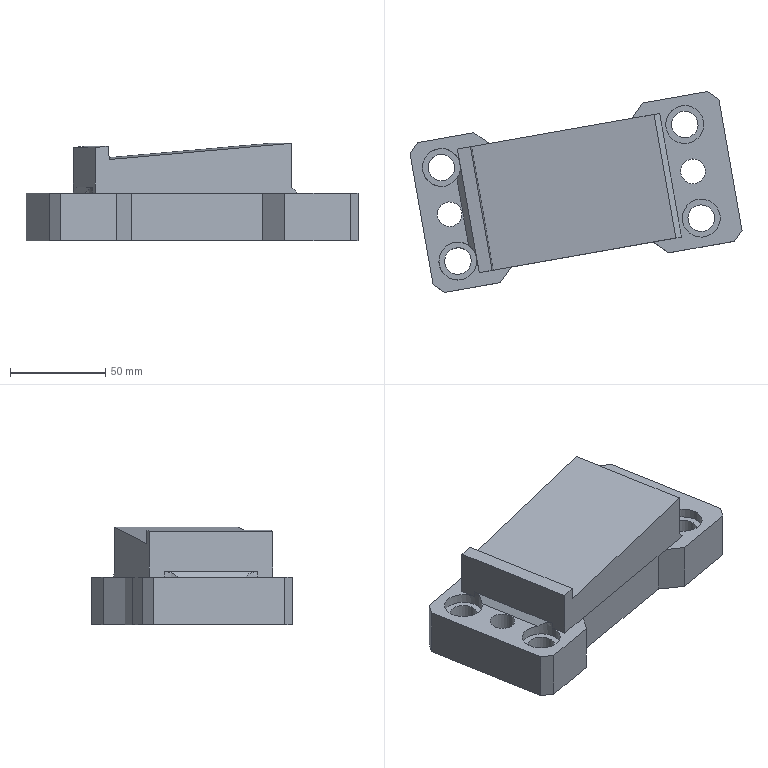Part | NX | features solid 2 | 1 solid | 44 faces | box 174.649 x 105.7 x 51.217 mm | volume 417191 mm3 | plane 34 | cylinder 10 | commonest cylinder face diameters 14 x4 20 x4 13 x2
STEP:
#1=CARTESIAN_POINT('',(1709.037,644.563,-70.));
#2=VERTEX_POINT('',#1);
#3=CARTESIAN_POINT('',(1694.265,641.959,-70.));
#4=VERTEX_POINT('',#3);
#5=CARTESIAN_POINT('',(1706.082,644.043,-70.));
#6=DIRECTION('',(-0.9848,-0.1736,0.));
#7=VECTOR('',#6,1000.);
#8=LINE('',#5,#7);
#9=EDGE_CURVE('',#2,#4,#8,.T.);
#10=ORIENTED_EDGE('',*,*,#9,.F.);
#11=CARTESIAN_POINT('',(1720.498,579.566,-70.));
#12=VERTEX_POINT('',#11);
#13=CARTESIAN_POINT('',(1714.767,612.065,-70.));
#14=DIRECTION('',(0.1736,-0.9848,0.));
#15=VECTOR('',#14,1000.);
#16=LINE('',#13,#15);
#17=EDGE_CURVE('',#2,#12,#16,.T.);
#18=ORIENTED_EDGE('',*,*,#17,.T.);
#19=CARTESIAN_POINT('',(1705.725,576.961,-70.));
#20=VERTEX_POINT('',#19);
#21=CARTESIAN_POINT('',(1717.543,579.045,-70.));
#22=DIRECTION('',(-0.9848,-0.1736,0.));
#23=VECTOR('',#22,1000.);
#24=LINE('',#21,#23);
#25=EDGE_CURVE('',#12,#20,#24,.T.);
#26=ORIENTED_EDGE('',*,*,#25,.T.);
#27=CARTESIAN_POINT('',(1713.835,571.283,-70.));
#28=VERTEX_POINT('',#27);
#29=CARTESIAN_POINT('',(1713.835,571.283,-70.));
#30=DIRECTION('',(-0.8192,0.5736,0.));
#31=VECTOR('',#30,1000.);
#32=LINE('',#29,#31);
#33=EDGE_CURVE('',#28,#20,#32,.T.);
#34=ORIENTED_EDGE('',*,*,#33,.F.);
#35=CARTESIAN_POINT('',(1748.303,577.361,-70.));
#36=VERTEX_POINT('',#35);
#37=CARTESIAN_POINT('',(1671.98,563.903,-70.));
#38=DIRECTION('',(-0.9848,-0.1736,0.));
#39=VECTOR('',#38,1000.);
#40=LINE('',#37,#39);
#41=EDGE_CURVE('',#36,#28,#40,.T.);
#42=ORIENTED_EDGE('',*,*,#41,.F.);
#43=CARTESIAN_POINT('',(1752.359,583.153,-70.));
#44=VERTEX_POINT('',#43);
#45=CARTESIAN_POINT('',(1733.094,555.64,-70.));
#46=DIRECTION('',(-0.5736,-0.8192,0.));
#47=VECTOR('',#46,1000.);
#48=LINE('',#45,#47);
#49=EDGE_CURVE('',#36,#44,#48,.F.);
#50=ORIENTED_EDGE('',*,*,#49,.T.);
#51=CARTESIAN_POINT('',(1740.203,652.09,-70.));
#52=VERTEX_POINT('',#51);
#53=CARTESIAN_POINT('',(1746.281,617.622,-70.));
#54=DIRECTION('',(0.1736,-0.9848,0.));
#55=VECTOR('',#54,1000.);
#56=LINE('',#53,#55);
#57=EDGE_CURVE('',#52,#44,#56,.T.);
#58=ORIENTED_EDGE('',*,*,#57,.F.);
#59=CARTESIAN_POINT('',(1734.411,656.146,-70.));
#60=VERTEX_POINT('',#59);
#61=CARTESIAN_POINT('',(1712.69,671.355,-70.));
#62=DIRECTION('',(0.8192,-0.5736,0.));
#63=VECTOR('',#62,1000.);
#64=LINE('',#61,#63);
#65=EDGE_CURVE('',#52,#60,#64,.F.);
#66=ORIENTED_EDGE('',*,*,#65,.T.);
#67=CARTESIAN_POINT('',(1699.943,650.068,-70.));
#68=VERTEX_POINT('',#67);
#69=CARTESIAN_POINT('',(1658.089,642.688,-70.));
#70=DIRECTION('',(0.9848,0.1736,0.));
#71=VECTOR('',#70,1000.);
#72=LINE('',#69,#71);
#73=EDGE_CURVE('',#68,#60,#72,.T.);
#74=ORIENTED_EDGE('',*,*,#73,.F.);
#75=CARTESIAN_POINT('',(1691.831,638.483,-70.));
#76=DIRECTION('',(0.5736,0.8192,0.));
#77=VECTOR('',#76,1000.);
#78=LINE('',#75,#77);
#79=EDGE_CURVE('',#4,#68,#78,.T.);
#80=ORIENTED_EDGE('',*,*,#79,.F.);
#81=EDGE_LOOP('',(#10,#18,#26,#34,#42,#50,#58,#66,#74,#80));
#82=FACE_BOUND('',#81,.T.);
#83=CARTESIAN_POINT('',(1721.078,587.792,-70.));
#84=VERTEX_POINT('',#83);
#85=CARTESIAN_POINT('',(1730.926,589.528,-70.));
#86=DIRECTION('',(0.,0.,1.));
#87=DIRECTION('',(-0.9848,-0.1736,0.));
#88=AXIS2_PLACEMENT_3D('',#85,#86,#87);
#89=CIRCLE('',#88,10.);
#90=EDGE_CURVE('',#84,#84,#89,.T.);
#91=ORIENTED_EDGE('',*,*,#90,.F.);
#92=EDGE_LOOP('',(#91));
#93=FACE_BOUND('',#92,.T.);
#94=CARTESIAN_POINT('',(1720.184,613.02,-70.));
#95=VERTEX_POINT('',#94);
#96=CARTESIAN_POINT('',(1726.585,614.149,-70.));
#97=DIRECTION('',(0.,0.,1.));
#98=DIRECTION('',(-0.9848,-0.1736,0.));
#99=AXIS2_PLACEMENT_3D('',#96,#97,#98);
#100=CIRCLE('',#99,6.5);
#101=EDGE_CURVE('',#95,#95,#100,.T.);
#102=ORIENTED_EDGE('',*,*,#101,.F.);
#103=EDGE_LOOP('',(#102));
#104=FACE_BOUND('',#103,.T.);
#105=CARTESIAN_POINT('',(1712.396,637.032,-70.));
#106=VERTEX_POINT('',#105);
#107=CARTESIAN_POINT('',(1722.244,638.769,-70.));
#108=DIRECTION('',(0.,0.,1.));
#109=DIRECTION('',(-0.9848,-0.1736,0.));
#110=AXIS2_PLACEMENT_3D('',#107,#108,#109);
#111=CIRCLE('',#110,10.);
#112=EDGE_CURVE('',#106,#106,#111,.T.);
#113=ORIENTED_EDGE('',*,*,#112,.F.);
#114=EDGE_LOOP('',(#113));
#115=FACE_BOUND('',#114,.T.);
#116=CARTESIAN_POINT('',(1665.034,603.296,-70.));
#117=DIRECTION('',(0.,0.,1.));
#118=DIRECTION('',(-0.9848,-0.1736,0.));
#119=AXIS2_PLACEMENT_3D('',#116,#117,#118);
#120=PLANE('',#119);
#121=ADVANCED_FACE('',(#82,#93,#104,#115),#120,.T.);
#122=CARTESIAN_POINT('',(1608.555,575.203,-70.));
#123=VERTEX_POINT('',#122);
#124=CARTESIAN_POINT('',(1612.749,568.691,-70.));
#125=VERTEX_POINT('',#124);
#126=CARTESIAN_POINT('',(1602.901,566.954,-70.));
#127=DIRECTION('',(0.,0.,1.));
#128=DIRECTION('',(-0.9848,-0.1736,0.));
#129=AXIS2_PLACEMENT_3D('',#126,#127,#128);
#130=CIRCLE('',#129,10.);
#131=EDGE_CURVE('',#123,#125,#130,.T.);
#132=ORIENTED_EDGE('',*,*,#131,.F.);
#133=CARTESIAN_POINT('',(1602.352,610.377,-70.));
#134=VERTEX_POINT('',#133);
#135=CARTESIAN_POINT('',(1601.112,617.41,-70.));
#136=DIRECTION('',(-0.1736,0.9848,0.));
#137=VECTOR('',#136,1000.);
#138=LINE('',#135,#137);
#139=EDGE_CURVE('',#123,#134,#138,.T.);
#140=ORIENTED_EDGE('',*,*,#139,.T.);
#141=CARTESIAN_POINT('',(1604.067,617.931,-70.));
#142=VERTEX_POINT('',#141);
#143=CARTESIAN_POINT('',(1594.219,616.195,-70.));
#144=DIRECTION('',(0.,0.,1.));
#145=DIRECTION('',(-0.9848,-0.1736,0.));
#146=AXIS2_PLACEMENT_3D('',#143,#144,#145);
#147=CIRCLE('',#146,10.);
#148=EDGE_CURVE('',#142,#134,#147,.T.);
#149=ORIENTED_EDGE('',*,*,#148,.F.);
#150=CARTESIAN_POINT('',(1602.678,625.809,-70.));
#151=VERTEX_POINT('',#150);
#152=CARTESIAN_POINT('',(1614.138,560.812,-70.));
#153=DIRECTION('',(-0.1736,0.9848,0.));
#154=VECTOR('',#153,1000.);
#155=LINE('',#152,#154);
#156=EDGE_CURVE('',#142,#151,#155,.T.);
#157=ORIENTED_EDGE('',*,*,#156,.T.);
#158=CARTESIAN_POINT('',(1619.419,628.762,-70.));
#159=VERTEX_POINT('',#158);
#160=CARTESIAN_POINT('',(1706.082,644.043,-70.));
#161=DIRECTION('',(-0.9848,-0.1736,0.));
#162=VECTOR('',#161,1000.);
#163=LINE('',#160,#162);
#164=EDGE_CURVE('',#159,#151,#163,.T.);
#165=ORIENTED_EDGE('',*,*,#164,.F.);
#166=CARTESIAN_POINT('',(1611.31,634.44,-70.));
#167=VERTEX_POINT('',#166);
#168=CARTESIAN_POINT('',(1622.895,626.328,-70.));
#169=DIRECTION('',(-0.8192,0.5736,0.));
#170=VECTOR('',#169,1000.);
#171=LINE('',#168,#170);
#172=EDGE_CURVE('',#159,#167,#171,.T.);
#173=ORIENTED_EDGE('',*,*,#172,.T.);
#174=CARTESIAN_POINT('',(1581.766,629.23,-70.));
#175=VERTEX_POINT('',#174);
#176=CARTESIAN_POINT('',(1658.089,642.688,-70.));
#177=DIRECTION('',(0.9848,0.1736,0.));
#178=VECTOR('',#177,1000.);
#179=LINE('',#176,#178);
#180=EDGE_CURVE('',#175,#167,#179,.T.);
#181=ORIENTED_EDGE('',*,*,#180,.F.);
#182=CARTESIAN_POINT('',(1577.71,623.438,-70.));
#183=VERTEX_POINT('',#182);
#184=CARTESIAN_POINT('',(1596.975,650.951,-70.));
#185=DIRECTION('',(0.5736,0.8192,0.));
#186=VECTOR('',#185,1000.);
#187=LINE('',#184,#186);
#188=EDGE_CURVE('',#175,#183,#187,.F.);
#189=ORIENTED_EDGE('',*,*,#188,.T.);
#190=CARTESIAN_POINT('',(1589.865,554.501,-70.));
#191=VERTEX_POINT('',#190);
#192=CARTESIAN_POINT('',(1583.788,588.97,-70.));
#193=DIRECTION('',(-0.1736,0.9848,0.));
#194=VECTOR('',#193,1000.);
#195=LINE('',#192,#194);
#196=EDGE_CURVE('',#191,#183,#195,.T.);
#197=ORIENTED_EDGE('',*,*,#196,.F.);
#198=CARTESIAN_POINT('',(1595.658,550.446,-70.));
#199=VERTEX_POINT('',#198);
#200=CARTESIAN_POINT('',(1617.379,535.236,-70.));
#201=DIRECTION('',(-0.8192,0.5736,0.));
#202=VECTOR('',#201,1000.);
#203=LINE('',#200,#202);
#204=EDGE_CURVE('',#191,#199,#203,.F.);
#205=ORIENTED_EDGE('',*,*,#204,.T.);
#206=CARTESIAN_POINT('',(1625.202,555.655,-70.));
#207=VERTEX_POINT('',#206);
#208=CARTESIAN_POINT('',(1671.98,563.903,-70.));
#209=DIRECTION('',(-0.9848,-0.1736,0.));
#210=VECTOR('',#209,1000.);
#211=LINE('',#208,#210);
#212=EDGE_CURVE('',#207,#199,#211,.T.);
#213=ORIENTED_EDGE('',*,*,#212,.F.);
#214=CARTESIAN_POINT('',(1630.88,563.764,-70.));
#215=VERTEX_POINT('',#214);
#216=CARTESIAN_POINT('',(1625.202,555.655,-70.));
#217=DIRECTION('',(0.5736,0.8192,0.));
#218=VECTOR('',#217,1000.);
#219=LINE('',#216,#218);
#220=EDGE_CURVE('',#207,#215,#219,.T.);
#221=ORIENTED_EDGE('',*,*,#220,.T.);
#222=CARTESIAN_POINT('',(1614.138,560.812,-70.));
#223=VERTEX_POINT('',#222);
#224=CARTESIAN_POINT('',(1717.543,579.045,-70.));
#225=DIRECTION('',(-0.9848,-0.1736,0.));
#226=VECTOR('',#225,1000.);
#227=LINE('',#224,#226);
#228=EDGE_CURVE('',#215,#223,#227,.T.);
#229=ORIENTED_EDGE('',*,*,#228,.T.);
#230=CARTESIAN_POINT('',(1614.138,560.812,-70.));
#231=DIRECTION('',(-0.1736,0.9848,0.));
#232=VECTOR('',#231,1000.);
#233=LINE('',#230,#232);
#234=EDGE_CURVE('',#223,#125,#233,.T.);
#235=ORIENTED_EDGE('',*,*,#234,.T.);
#236=EDGE_LOOP('',(#132,#140,#149,#157,#165,#173,#181,#189,#197,#205,#213,#221,#229,#235));
#237=FACE_BOUND('',#236,.T.);
#238=CARTESIAN_POINT('',(1592.159,590.446,-70.));
#239=VERTEX_POINT('',#238);
#240=CARTESIAN_POINT('',(1598.56,591.574,-70.));
#241=DIRECTION('',(0.,0.,1.));
#242=DIRECTION('',(-0.9848,-0.1736,0.));
#243=AXIS2_PLACEMENT_3D('',#240,#241,#242);
#244=CIRCLE('',#243,6.5);
#245=EDGE_CURVE('',#239,#239,#244,.T.);
#246=ORIENTED_EDGE('',*,*,#245,.F.);
#247=EDGE_LOOP('',(#246));
#248=FACE_BOUND('',#247,.T.);
#249=CARTESIAN_POINT('',(1665.034,603.296,-70.));
#250=DIRECTION('',(0.,0.,1.));
#251=DIRECTION('',(-0.9848,-0.1736,0.));
#252=AXIS2_PLACEMENT_3D('',#249,#250,#251);
#253=PLANE('',#252);
#254=ADVANCED_FACE('',(#237,#248),#253,.T.);
#255=CARTESIAN_POINT('',(1724.032,588.313,-95.));
#256=VERTEX_POINT('',#255);
#257=CARTESIAN_POINT('',(1730.926,589.528,-95.));
#258=DIRECTION('',(0.,0.,1.));
#259=DIRECTION('',(-0.9848,-0.1736,0.));
#260=AXIS2_PLACEMENT_3D('',#257,#258,#259);
#261=CIRCLE('',#260,7.);
#262=EDGE_CURVE('',#256,#256,#261,.T.);
#263=ORIENTED_EDGE('',*,*,#262,.F.);
#264=EDGE_LOOP('',(#263));
#265=FACE_BOUND('',#264,.T.);
#266=CARTESIAN_POINT('',(1737.82,590.744,-75.));
#267=VERTEX_POINT('',#266);
#268=CARTESIAN_POINT('',(1730.926,589.528,-75.));
#269=DIRECTION('',(0.,0.,1.));
#270=DIRECTION('',(0.9848,0.1736,0.));
#271=AXIS2_PLACEMENT_3D('',#268,#269,#270);
#272=CIRCLE('',#271,7.);
#273=EDGE_CURVE('',#267,#267,#272,.T.);
#274=ORIENTED_EDGE('',*,*,#273,.T.);
#275=EDGE_LOOP('',(#274));
#276=FACE_BOUND('',#275,.T.);
#277=CARTESIAN_POINT('',(1730.926,589.528,-70.));
#278=DIRECTION('',(0.,0.,-1.));
#279=DIRECTION('',(0.1736,-0.9848,0.));
#280=AXIS2_PLACEMENT_3D('',#277,#278,#279);
#281=CYLINDRICAL_SURFACE('',#280,7.);
#282=ADVANCED_FACE('',(#265,#276),#281,.F.);
#283=CARTESIAN_POINT('',(1715.35,637.553,-95.));
#284=VERTEX_POINT('',#283);
#285=CARTESIAN_POINT('',(1722.244,638.769,-95.));
#286=DIRECTION('',(0.,0.,1.));
#287=DIRECTION('',(-0.9848,-0.1736,0.));
#288=AXIS2_PLACEMENT_3D('',#285,#286,#287);
#289=CIRCLE('',#288,7.);
#290=EDGE_CURVE('',#284,#284,#289,.T.);
#291=ORIENTED_EDGE('',*,*,#290,.F.);
#292=EDGE_LOOP('',(#291));
#293=FACE_BOUND('',#292,.T.);
#294=CARTESIAN_POINT('',(1729.137,639.984,-75.));
#295=VERTEX_POINT('',#294);
#296=CARTESIAN_POINT('',(1722.244,638.769,-75.));
#297=DIRECTION('',(0.,0.,1.));
#298=DIRECTION('',(0.9848,0.1736,0.));
#299=AXIS2_PLACEMENT_3D('',#296,#297,#298);
#300=CIRCLE('',#299,7.);
#301=EDGE_CURVE('',#295,#295,#300,.T.);
#302=ORIENTED_EDGE('',*,*,#301,.T.);
#303=EDGE_LOOP('',(#302));
#304=FACE_BOUND('',#303,.T.);
#305=CARTESIAN_POINT('',(1722.244,638.769,-70.));
#306=DIRECTION('',(0.,0.,-1.));
#307=DIRECTION('',(0.1736,-0.9848,0.));
#308=AXIS2_PLACEMENT_3D('',#305,#306,#307);
#309=CYLINDRICAL_SURFACE('',#308,7.);
#310=ADVANCED_FACE('',(#293,#304),#309,.F.);
#311=CARTESIAN_POINT('',(1587.325,614.979,-95.));
#312=VERTEX_POINT('',#311);
#313=CARTESIAN_POINT('',(1594.219,616.195,-95.));
#314=DIRECTION('',(0.,0.,1.));
#315=DIRECTION('',(-0.9848,-0.1736,0.));
#316=AXIS2_PLACEMENT_3D('',#313,#314,#315);
#317=CIRCLE('',#316,7.);
#318=EDGE_CURVE('',#312,#312,#317,.T.);
#319=ORIENTED_EDGE('',*,*,#318,.F.);
#320=EDGE_LOOP('',(#319));
#321=FACE_BOUND('',#320,.T.);
#322=CARTESIAN_POINT('',(1601.112,617.41,-75.));
#323=VERTEX_POINT('',#322);
#324=CARTESIAN_POINT('',(1594.219,616.195,-75.));
#325=DIRECTION('',(0.,0.,1.));
#326=DIRECTION('',(0.9848,0.1736,0.));
#327=AXIS2_PLACEMENT_3D('',#324,#325,#326);
#328=CIRCLE('',#327,7.);
#329=EDGE_CURVE('',#323,#323,#328,.T.);
#330=ORIENTED_EDGE('',*,*,#329,.T.);
#331=EDGE_LOOP('',(#330));
#332=FACE_BOUND('',#331,.T.);
#333=CARTESIAN_POINT('',(1594.219,616.195,-70.));
#334=DIRECTION('',(0.,0.,-1.));
#335=DIRECTION('',(0.1736,-0.9848,0.));
#336=AXIS2_PLACEMENT_3D('',#333,#334,#335);
#337=CYLINDRICAL_SURFACE('',#336,7.);
#338=ADVANCED_FACE('',(#321,#332),#337,.F.);
#339=CARTESIAN_POINT('',(1596.007,565.739,-95.));
#340=VERTEX_POINT('',#339);
#341=CARTESIAN_POINT('',(1602.901,566.954,-95.));
#342=DIRECTION('',(0.,0.,1.));
#343=DIRECTION('',(-0.9848,-0.1736,0.));
#344=AXIS2_PLACEMENT_3D('',#341,#342,#343);
#345=CIRCLE('',#344,7.);
#346=EDGE_CURVE('',#340,#340,#345,.T.);
#347=ORIENTED_EDGE('',*,*,#346,.F.);
#348=EDGE_LOOP('',(#347));
#349=FACE_BOUND('',#348,.T.);
#350=CARTESIAN_POINT('',(1609.795,568.17,-75.));
#351=VERTEX_POINT('',#350);
#352=CARTESIAN_POINT('',(1602.901,566.954,-75.));
#353=DIRECTION('',(0.,0.,1.));
#354=DIRECTION('',(0.9848,0.1736,0.));
#355=AXIS2_PLACEMENT_3D('',#352,#353,#354);
#356=CIRCLE('',#355,7.);
#357=EDGE_CURVE('',#351,#351,#356,.T.);
#358=ORIENTED_EDGE('',*,*,#357,.T.);
#359=EDGE_LOOP('',(#358));
#360=FACE_BOUND('',#359,.T.);
#361=CARTESIAN_POINT('',(1602.901,566.954,-70.));
#362=DIRECTION('',(0.,0.,-1.));
#363=DIRECTION('',(0.1736,-0.9848,0.));
#364=AXIS2_PLACEMENT_3D('',#361,#362,#363);
#365=CYLINDRICAL_SURFACE('',#364,7.);
#366=ADVANCED_FACE('',(#349,#360),#365,.F.);
#367=CARTESIAN_POINT('',(1720.184,613.02,-95.));
#368=VERTEX_POINT('',#367);
#369=CARTESIAN_POINT('',(1726.585,614.149,-95.));
#370=DIRECTION('',(0.,0.,1.));
#371=DIRECTION('',(-0.9848,-0.1736,0.));
#372=AXIS2_PLACEMENT_3D('',#369,#370,#371);
#373=CIRCLE('',#372,6.5);
#374=EDGE_CURVE('',#368,#368,#373,.T.);
#375=ORIENTED_EDGE('',*,*,#374,.T.);
#376=EDGE_LOOP('',(#375));
#377=FACE_BOUND('',#376,.T.);
#378=ORIENTED_EDGE('',*,*,#318,.T.);
#379=EDGE_LOOP('',(#378));
#380=FACE_BOUND('',#379,.T.);
#381=ORIENTED_EDGE('',*,*,#346,.T.);
#382=EDGE_LOOP('',(#381));
#383=FACE_BOUND('',#382,.T.);
#384=CARTESIAN_POINT('',(1595.658,550.446,-95.));
#385=VERTEX_POINT('',#384);
#386=CARTESIAN_POINT('',(1625.202,555.655,-95.));
#387=VERTEX_POINT('',#386);
#388=CARTESIAN_POINT('',(1671.98,563.903,-95.));
#389=DIRECTION('',(0.9848,0.1736,0.));
#390=VECTOR('',#389,1000.);
#391=LINE('',#388,#390);
#392=EDGE_CURVE('',#385,#387,#391,.T.);
#393=ORIENTED_EDGE('',*,*,#392,.F.);
#394=CARTESIAN_POINT('',(1589.865,554.501,-95.));
#395=VERTEX_POINT('',#394);
#396=CARTESIAN_POINT('',(1617.379,535.236,-95.));
#397=DIRECTION('',(0.8192,-0.5736,0.));
#398=VECTOR('',#397,1000.);
#399=LINE('',#396,#398);
#400=EDGE_CURVE('',#385,#395,#399,.F.);
#401=ORIENTED_EDGE('',*,*,#400,.T.);
#402=CARTESIAN_POINT('',(1577.71,623.438,-95.));
#403=VERTEX_POINT('',#402);
#404=CARTESIAN_POINT('',(1583.788,588.97,-95.));
#405=DIRECTION('',(0.1736,-0.9848,0.));
#406=VECTOR('',#405,1000.);
#407=LINE('',#404,#406);
#408=EDGE_CURVE('',#403,#395,#407,.T.);
#409=ORIENTED_EDGE('',*,*,#408,.F.);
#410=CARTESIAN_POINT('',(1581.766,629.23,-95.));
#411=VERTEX_POINT('',#410);
#412=CARTESIAN_POINT('',(1596.975,650.951,-95.));
#413=DIRECTION('',(-0.5736,-0.8192,0.));
#414=VECTOR('',#413,1000.);
#415=LINE('',#412,#414);
#416=EDGE_CURVE('',#403,#411,#415,.F.);
#417=ORIENTED_EDGE('',*,*,#416,.T.);
#418=CARTESIAN_POINT('',(1611.31,634.44,-95.));
#419=VERTEX_POINT('',#418);
#420=CARTESIAN_POINT('',(1658.089,642.688,-95.));
#421=DIRECTION('',(-0.9848,-0.1736,0.));
#422=VECTOR('',#421,1000.);
#423=LINE('',#420,#422);
#424=EDGE_CURVE('',#419,#411,#423,.T.);
#425=ORIENTED_EDGE('',*,*,#424,.F.);
#426=CARTESIAN_POINT('',(1622.895,626.328,-95.));
#427=VERTEX_POINT('',#426);
#428=CARTESIAN_POINT('',(1622.895,626.328,-95.));
#429=DIRECTION('',(-0.8192,0.5736,0.));
#430=VECTOR('',#429,1000.);
#431=LINE('',#428,#430);
#432=EDGE_CURVE('',#427,#419,#431,.T.);
#433=ORIENTED_EDGE('',*,*,#432,.F.);
#434=CARTESIAN_POINT('',(1691.831,638.483,-95.));
#435=VERTEX_POINT('',#434);
#436=CARTESIAN_POINT('',(1691.831,638.483,-95.));
#437=DIRECTION('',(-0.9848,-0.1736,0.));
#438=VECTOR('',#437,1000.);
#439=LINE('',#436,#438);
#440=EDGE_CURVE('',#435,#427,#439,.T.);
#441=ORIENTED_EDGE('',*,*,#440,.F.);
#442=CARTESIAN_POINT('',(1699.943,650.068,-95.));
#443=VERTEX_POINT('',#442);
#444=CARTESIAN_POINT('',(1691.831,638.483,-95.));
#445=DIRECTION('',(0.5736,0.8192,0.));
#446=VECTOR('',#445,1000.);
#447=LINE('',#444,#446);
#448=EDGE_CURVE('',#435,#443,#447,.T.);
#449=ORIENTED_EDGE('',*,*,#448,.T.);
#450=CARTESIAN_POINT('',(1734.411,656.146,-95.));
#451=VERTEX_POINT('',#450);
#452=CARTESIAN_POINT('',(1658.089,642.688,-95.));
#453=DIRECTION('',(-0.9848,-0.1736,0.));
#454=VECTOR('',#453,1000.);
#455=LINE('',#452,#454);
#456=EDGE_CURVE('',#451,#443,#455,.T.);
#457=ORIENTED_EDGE('',*,*,#456,.F.);
#458=CARTESIAN_POINT('',(1740.203,652.09,-95.));
#459=VERTEX_POINT('',#458);
#460=CARTESIAN_POINT('',(1712.69,671.355,-95.));
#461=DIRECTION('',(-0.8192,0.5736,0.));
#462=VECTOR('',#461,1000.);
#463=LINE('',#460,#462);
#464=EDGE_CURVE('',#451,#459,#463,.F.);
#465=ORIENTED_EDGE('',*,*,#464,.T.);
#466=CARTESIAN_POINT('',(1752.359,583.153,-95.));
#467=VERTEX_POINT('',#466);
#468=CARTESIAN_POINT('',(1746.281,617.622,-95.));
#469=DIRECTION('',(-0.1736,0.9848,0.));
#470=VECTOR('',#469,1000.);
#471=LINE('',#468,#470);
#472=EDGE_CURVE('',#467,#459,#471,.T.);
#473=ORIENTED_EDGE('',*,*,#472,.F.);
#474=CARTESIAN_POINT('',(1748.303,577.361,-95.));
#475=VERTEX_POINT('',#474);
#476=CARTESIAN_POINT('',(1733.094,555.64,-95.));
#477=DIRECTION('',(0.5736,0.8192,0.));
#478=VECTOR('',#477,1000.);
#479=LINE('',#476,#478);
#480=EDGE_CURVE('',#467,#475,#479,.F.);
#481=ORIENTED_EDGE('',*,*,#480,.T.);
#482=CARTESIAN_POINT('',(1713.835,571.283,-95.));
#483=VERTEX_POINT('',#482);
#484=CARTESIAN_POINT('',(1671.98,563.903,-95.));
#485=DIRECTION('',(0.9848,0.1736,0.));
#486=VECTOR('',#485,1000.);
#487=LINE('',#484,#486);
#488=EDGE_CURVE('',#483,#475,#487,.T.);
#489=ORIENTED_EDGE('',*,*,#488,.F.);
#490=CARTESIAN_POINT('',(1702.25,579.395,-95.));
#491=VERTEX_POINT('',#490);
#492=CARTESIAN_POINT('',(1713.835,571.283,-95.));
#493=DIRECTION('',(-0.8192,0.5736,0.));
#494=VECTOR('',#493,1000.);
#495=LINE('',#492,#494);
#496=EDGE_CURVE('',#483,#491,#495,.T.);
#497=ORIENTED_EDGE('',*,*,#496,.T.);
#498=CARTESIAN_POINT('',(1633.314,567.24,-95.));
#499=VERTEX_POINT('',#498);
#500=CARTESIAN_POINT('',(1702.25,579.395,-95.));
#501=DIRECTION('',(-0.9848,-0.1736,0.));
#502=VECTOR('',#501,1000.);
#503=LINE('',#500,#502);
#504=EDGE_CURVE('',#491,#499,#503,.T.);
#505=ORIENTED_EDGE('',*,*,#504,.T.);
#506=CARTESIAN_POINT('',(1625.202,555.655,-95.));
#507=DIRECTION('',(0.5736,0.8192,0.));
#508=VECTOR('',#507,1000.);
#509=LINE('',#506,#508);
#510=EDGE_CURVE('',#387,#499,#509,.T.);
#511=ORIENTED_EDGE('',*,*,#510,.F.);
#512=EDGE_LOOP('',(#393,#401,#409,#417,#425,#433,#441,#449,#457,#465,#473,#481,#489,#497,#505,#511));
#513=FACE_BOUND('',#512,.T.);
#514=CARTESIAN_POINT('',(1592.159,590.446,-95.));
#515=VERTEX_POINT('',#514);
#516=CARTESIAN_POINT('',(1598.56,591.574,-95.));
#517=DIRECTION('',(0.,0.,1.));
#518=DIRECTION('',(-0.9848,-0.1736,0.));
#519=AXIS2_PLACEMENT_3D('',#516,#517,#518);
#520=CIRCLE('',#519,6.5);
#521=EDGE_CURVE('',#515,#515,#520,.T.);
#522=ORIENTED_EDGE('',*,*,#521,.T.);
#523=EDGE_LOOP('',(#522));
#524=FACE_BOUND('',#523,.T.);
#525=ORIENTED_EDGE('',*,*,#262,.T.);
#526=EDGE_LOOP('',(#525));
#527=FACE_BOUND('',#526,.T.);
#528=ORIENTED_EDGE('',*,*,#290,.T.);
#529=EDGE_LOOP('',(#528));
#530=FACE_BOUND('',#529,.T.);
#531=CARTESIAN_POINT('',(1665.034,603.296,-95.));
#532=DIRECTION('',(0.,0.,-1.));
#533=DIRECTION('',(0.9848,0.1736,0.));
#534=AXIS2_PLACEMENT_3D('',#531,#532,#533);
#535=PLANE('',#534);
#536=ADVANCED_FACE('',(#377,#380,#383,#513,#524,#527,#530),#535,.T.);
#537=ORIENTED_EDGE('',*,*,#73,.T.);
#538=CARTESIAN_POINT('',(1734.411,656.146,-95.));
#539=DIRECTION('',(0.,0.,-1.));
#540=VECTOR('',#539,1000.);
#541=LINE('',#538,#540);
#542=EDGE_CURVE('',#60,#451,#541,.T.);
#543=ORIENTED_EDGE('',*,*,#542,.T.);
#544=ORIENTED_EDGE('',*,*,#456,.T.);
#545=CARTESIAN_POINT('',(1699.943,650.068,-70.));
#546=DIRECTION('',(0.,0.,-1.));
#547=VECTOR('',#546,1000.);
#548=LINE('',#545,#547);
#549=EDGE_CURVE('',#68,#443,#548,.T.);
#550=ORIENTED_EDGE('',*,*,#549,.F.);
#551=EDGE_LOOP('',(#537,#543,#544,#550));
#552=FACE_BOUND('',#551,.T.);
#553=CARTESIAN_POINT('',(1658.089,642.688,-95.));
#554=DIRECTION('',(-0.1736,0.9848,0.));
#555=DIRECTION('',(0.,0.,-1.));
#556=AXIS2_PLACEMENT_3D('',#553,#554,#555);
#557=PLANE('',#556);
#558=ADVANCED_FACE('',(#552),#557,.T.);
#559=ORIENTED_EDGE('',*,*,#488,.T.);
#560=CARTESIAN_POINT('',(1748.303,577.361,-95.));
#561=DIRECTION('',(0.,0.,1.));
#562=VECTOR('',#561,1000.);
#563=LINE('',#560,#562);
#564=EDGE_CURVE('',#475,#36,#563,.T.);
#565=ORIENTED_EDGE('',*,*,#564,.T.);
#566=ORIENTED_EDGE('',*,*,#41,.T.);
#567=CARTESIAN_POINT('',(1713.835,571.283,-70.));
#568=DIRECTION('',(0.,0.,-1.));
#569=VECTOR('',#568,1000.);
#570=LINE('',#567,#569);
#571=EDGE_CURVE('',#28,#483,#570,.T.);
#572=ORIENTED_EDGE('',*,*,#571,.T.);
#573=EDGE_LOOP('',(#559,#565,#566,#572));
#574=FACE_BOUND('',#573,.T.);
#575=CARTESIAN_POINT('',(1671.98,563.903,-95.));
#576=DIRECTION('',(0.1736,-0.9848,0.));
#577=DIRECTION('',(0.,0.,1.));
#578=AXIS2_PLACEMENT_3D('',#575,#576,#577);
#579=PLANE('',#578);
#580=ADVANCED_FACE('',(#574),#579,.T.);
#581=ORIENTED_EDGE('',*,*,#424,.T.);
#582=CARTESIAN_POINT('',(1581.766,629.23,-95.));
#583=DIRECTION('',(0.,0.,1.));
#584=VECTOR('',#583,1000.);
#585=LINE('',#582,#584);
#586=EDGE_CURVE('',#411,#175,#585,.T.);
#587=ORIENTED_EDGE('',*,*,#586,.T.);
#588=ORIENTED_EDGE('',*,*,#180,.T.);
#589=CARTESIAN_POINT('',(1611.31,634.44,-70.));
#590=DIRECTION('',(0.,0.,-1.));
#591=VECTOR('',#590,1000.);
#592=LINE('',#589,#591);
#593=EDGE_CURVE('',#167,#419,#592,.T.);
#594=ORIENTED_EDGE('',*,*,#593,.T.);
#595=EDGE_LOOP('',(#581,#587,#588,#594));
#596=FACE_BOUND('',#595,.T.);
#597=CARTESIAN_POINT('',(1658.089,642.688,-95.));
#598=DIRECTION('',(-0.1736,0.9848,0.));
#599=DIRECTION('',(0.,0.,-1.));
#600=AXIS2_PLACEMENT_3D('',#597,#598,#599);
#601=PLANE('',#600);
#602=ADVANCED_FACE('',(#596),#601,.T.);
#603=ORIENTED_EDGE('',*,*,#472,.T.);
#604=CARTESIAN_POINT('',(1740.203,652.09,-95.));
#605=DIRECTION('',(0.,0.,1.));
#606=VECTOR('',#605,1000.);
#607=LINE('',#604,#606);
#608=EDGE_CURVE('',#459,#52,#607,.T.);
#609=ORIENTED_EDGE('',*,*,#608,.T.);
#610=ORIENTED_EDGE('',*,*,#57,.T.);
#611=CARTESIAN_POINT('',(1752.359,583.153,-95.));
#612=DIRECTION('',(0.,0.,-1.));
#613=VECTOR('',#612,1000.);
#614=LINE('',#611,#613);
#615=EDGE_CURVE('',#44,#467,#614,.T.);
#616=ORIENTED_EDGE('',*,*,#615,.T.);
#617=EDGE_LOOP('',(#603,#609,#610,#616));
#618=FACE_BOUND('',#617,.T.);
#619=CARTESIAN_POINT('',(1746.281,617.622,-95.));
#620=DIRECTION('',(0.9848,0.1736,0.));
#621=DIRECTION('',(0.,0.,1.));
#622=AXIS2_PLACEMENT_3D('',#619,#620,#621);
#623=PLANE('',#622);
#624=ADVANCED_FACE('',(#618),#623,.T.);
#625=ORIENTED_EDGE('',*,*,#212,.T.);
#626=CARTESIAN_POINT('',(1595.658,550.446,-95.));
#627=DIRECTION('',(0.,0.,-1.));
#628=VECTOR('',#627,1000.);
#629=LINE('',#626,#628);
#630=EDGE_CURVE('',#199,#385,#629,.T.);
#631=ORIENTED_EDGE('',*,*,#630,.T.);
#632=ORIENTED_EDGE('',*,*,#392,.T.);
#633=CARTESIAN_POINT('',(1625.202,555.655,-70.));
#634=DIRECTION('',(0.,0.,-1.));
#635=VECTOR('',#634,1000.);
#636=LINE('',#633,#635);
#637=EDGE_CURVE('',#207,#387,#636,.T.);
#638=ORIENTED_EDGE('',*,*,#637,.F.);
#639=EDGE_LOOP('',(#625,#631,#632,#638));
#640=FACE_BOUND('',#639,.T.);
#641=CARTESIAN_POINT('',(1671.98,563.903,-95.));
#642=DIRECTION('',(0.1736,-0.9848,0.));
#643=DIRECTION('',(0.,0.,1.));
#644=AXIS2_PLACEMENT_3D('',#641,#642,#643);
#645=PLANE('',#644);
#646=ADVANCED_FACE('',(#640),#645,.T.);
#647=ORIENTED_EDGE('',*,*,#408,.T.);
#648=CARTESIAN_POINT('',(1589.865,554.501,-95.));
#649=DIRECTION('',(0.,0.,1.));
#650=VECTOR('',#649,1000.);
#651=LINE('',#648,#650);
#652=EDGE_CURVE('',#395,#191,#651,.T.);
#653=ORIENTED_EDGE('',*,*,#652,.T.);
#654=ORIENTED_EDGE('',*,*,#196,.T.);
#655=CARTESIAN_POINT('',(1577.71,623.438,-95.));
#656=DIRECTION('',(0.,0.,-1.));
#657=VECTOR('',#656,1000.);
#658=LINE('',#655,#657);
#659=EDGE_CURVE('',#183,#403,#658,.T.);
#660=ORIENTED_EDGE('',*,*,#659,.T.);
#661=EDGE_LOOP('',(#647,#653,#654,#660));
#662=FACE_BOUND('',#661,.T.);
#663=CARTESIAN_POINT('',(1583.788,588.97,-95.));
#664=DIRECTION('',(-0.9848,-0.1736,0.));
#665=DIRECTION('',(0.,0.,-1.));
#666=AXIS2_PLACEMENT_3D('',#663,#664,#665);
#667=PLANE('',#666);
#668=ADVANCED_FACE('',(#662),#667,.T.);
#669=ORIENTED_EDGE('',*,*,#510,.T.);
#670=CARTESIAN_POINT('',(1633.314,567.24,-70.));
#671=VERTEX_POINT('',#670);
#672=CARTESIAN_POINT('',(1633.314,567.24,-70.));
#673=DIRECTION('',(0.,0.,-1.));
#674=VECTOR('',#673,1000.);
#675=LINE('',#672,#674);
#676=EDGE_CURVE('',#671,#499,#675,.T.);
#677=ORIENTED_EDGE('',*,*,#676,.F.);
#678=CARTESIAN_POINT('',(1625.202,555.655,-70.));
#679=DIRECTION('',(0.5736,0.8192,0.));
#680=VECTOR('',#679,1000.);
#681=LINE('',#678,#680);
#682=EDGE_CURVE('',#215,#671,#681,.T.);
#683=ORIENTED_EDGE('',*,*,#682,.F.);
#684=ORIENTED_EDGE('',*,*,#220,.F.);
#685=ORIENTED_EDGE('',*,*,#637,.T.);
#686=EDGE_LOOP('',(#669,#677,#683,#684,#685));
#687=FACE_BOUND('',#686,.T.);
#688=CARTESIAN_POINT('',(1625.202,555.655,-70.));
#689=DIRECTION('',(-0.8192,0.5736,0.));
#690=DIRECTION('',(-0.5736,-0.8192,0.));
#691=AXIS2_PLACEMENT_3D('',#688,#689,#690);
#692=PLANE('',#691);
#693=ADVANCED_FACE('',(#687),#692,.F.);
#694=ORIENTED_EDGE('',*,*,#504,.F.);
#695=CARTESIAN_POINT('',(1702.25,579.395,-70.));
#696=VERTEX_POINT('',#695);
#697=CARTESIAN_POINT('',(1702.25,579.395,-70.));
#698=DIRECTION('',(0.,0.,-1.));
#699=VECTOR('',#698,1000.);
#700=LINE('',#697,#699);
#701=EDGE_CURVE('',#696,#491,#700,.T.);
#702=ORIENTED_EDGE('',*,*,#701,.F.);
#703=CARTESIAN_POINT('',(1702.25,579.395,-70.));
#704=DIRECTION('',(-0.9848,-0.1736,0.));
#705=VECTOR('',#704,1000.);
#706=LINE('',#703,#705);
#707=EDGE_CURVE('',#696,#671,#706,.T.);
#708=ORIENTED_EDGE('',*,*,#707,.T.);
#709=ORIENTED_EDGE('',*,*,#676,.T.);
#710=EDGE_LOOP('',(#694,#702,#708,#709));
#711=FACE_BOUND('',#710,.T.);
#712=CARTESIAN_POINT('',(1702.25,579.395,-70.));
#713=DIRECTION('',(0.1736,-0.9848,0.));
#714=DIRECTION('',(0.9848,0.1736,0.));
#715=AXIS2_PLACEMENT_3D('',#712,#713,#714);
#716=PLANE('',#715);
#717=ADVANCED_FACE('',(#711),#716,.T.);
#718=ORIENTED_EDGE('',*,*,#496,.F.);
#719=ORIENTED_EDGE('',*,*,#571,.F.);
#720=ORIENTED_EDGE('',*,*,#33,.T.);
#721=CARTESIAN_POINT('',(1713.835,571.283,-70.));
#722=DIRECTION('',(-0.8192,0.5736,0.));
#723=VECTOR('',#722,1000.);
#724=LINE('',#721,#723);
#725=EDGE_CURVE('',#20,#696,#724,.T.);
#726=ORIENTED_EDGE('',*,*,#725,.T.);
#727=ORIENTED_EDGE('',*,*,#701,.T.);
#728=EDGE_LOOP('',(#718,#719,#720,#726,#727));
#729=FACE_BOUND('',#728,.T.);
#730=CARTESIAN_POINT('',(1713.835,571.283,-70.));
#731=DIRECTION('',(-0.5736,-0.8192,0.));
#732=DIRECTION('',(0.8192,-0.5736,0.));
#733=AXIS2_PLACEMENT_3D('',#730,#731,#732);
#734=PLANE('',#733);
#735=ADVANCED_FACE('',(#729),#734,.T.);
#736=ORIENTED_EDGE('',*,*,#432,.T.);
#737=ORIENTED_EDGE('',*,*,#593,.F.);
#738=ORIENTED_EDGE('',*,*,#172,.F.);
#739=CARTESIAN_POINT('',(1622.895,626.328,-70.));
#740=VERTEX_POINT('',#739);
#741=CARTESIAN_POINT('',(1622.895,626.328,-70.));
#742=DIRECTION('',(-0.8192,0.5736,0.));
#743=VECTOR('',#742,1000.);
#744=LINE('',#741,#743);
#745=EDGE_CURVE('',#740,#159,#744,.T.);
#746=ORIENTED_EDGE('',*,*,#745,.F.);
#747=CARTESIAN_POINT('',(1622.895,626.328,-70.));
#748=DIRECTION('',(0.,0.,-1.));
#749=VECTOR('',#748,1000.);
#750=LINE('',#747,#749);
#751=EDGE_CURVE('',#740,#427,#750,.T.);
#752=ORIENTED_EDGE('',*,*,#751,.T.);
#753=EDGE_LOOP('',(#736,#737,#738,#746,#752));
#754=FACE_BOUND('',#753,.T.);
#755=CARTESIAN_POINT('',(1622.895,626.328,-70.));
#756=DIRECTION('',(-0.5736,-0.8192,0.));
#757=DIRECTION('',(0.8192,-0.5736,0.));
#758=AXIS2_PLACEMENT_3D('',#755,#756,#757);
#759=PLANE('',#758);
#760=ADVANCED_FACE('',(#754),#759,.F.);
#761=ORIENTED_EDGE('',*,*,#448,.F.);
#762=CARTESIAN_POINT('',(1691.831,638.483,-70.));
#763=VERTEX_POINT('',#762);
#764=CARTESIAN_POINT('',(1691.831,638.483,-70.));
#765=DIRECTION('',(0.,0.,-1.));
#766=VECTOR('',#765,1000.);
#767=LINE('',#764,#766);
#768=EDGE_CURVE('',#763,#435,#767,.T.);
#769=ORIENTED_EDGE('',*,*,#768,.F.);
#770=CARTESIAN_POINT('',(1691.831,638.483,-70.));
#771=DIRECTION('',(0.5736,0.8192,0.));
#772=VECTOR('',#771,1000.);
#773=LINE('',#770,#772);
#774=EDGE_CURVE('',#763,#4,#773,.T.);
#775=ORIENTED_EDGE('',*,*,#774,.T.);
#776=ORIENTED_EDGE('',*,*,#79,.T.);
#777=ORIENTED_EDGE('',*,*,#549,.T.);
#778=EDGE_LOOP('',(#761,#769,#775,#776,#777));
#779=FACE_BOUND('',#778,.T.);
#780=CARTESIAN_POINT('',(1691.831,638.483,-70.));
#781=DIRECTION('',(-0.8192,0.5736,0.));
#782=DIRECTION('',(-0.5736,-0.8192,0.));
#783=AXIS2_PLACEMENT_3D('',#780,#781,#782);
#784=PLANE('',#783);
#785=ADVANCED_FACE('',(#779),#784,.T.);
#786=ORIENTED_EDGE('',*,*,#440,.T.);
#787=ORIENTED_EDGE('',*,*,#751,.F.);
#788=CARTESIAN_POINT('',(1691.831,638.483,-70.));
#789=DIRECTION('',(-0.9848,-0.1736,0.));
#790=VECTOR('',#789,1000.);
#791=LINE('',#788,#790);
#792=EDGE_CURVE('',#763,#740,#791,.T.);
#793=ORIENTED_EDGE('',*,*,#792,.F.);
#794=ORIENTED_EDGE('',*,*,#768,.T.);
#795=EDGE_LOOP('',(#786,#787,#793,#794));
#796=FACE_BOUND('',#795,.T.);
#797=CARTESIAN_POINT('',(1691.831,638.483,-70.));
#798=DIRECTION('',(0.1736,-0.9848,0.));
#799=DIRECTION('',(0.9848,0.1736,0.));
#800=AXIS2_PLACEMENT_3D('',#797,#798,#799);
#801=PLANE('',#800);
#802=ADVANCED_FACE('',(#796),#801,.F.);
#803=ORIENTED_EDGE('',*,*,#245,.T.);
#804=EDGE_LOOP('',(#803));
#805=FACE_BOUND('',#804,.T.);
#806=ORIENTED_EDGE('',*,*,#521,.F.);
#807=EDGE_LOOP('',(#806));
#808=FACE_BOUND('',#807,.T.);
#809=CARTESIAN_POINT('',(1598.56,591.574,-70.));
#810=DIRECTION('',(0.,0.,-1.));
#811=DIRECTION('',(0.1736,-0.9848,0.));
#812=AXIS2_PLACEMENT_3D('',#809,#810,#811);
#813=CYLINDRICAL_SURFACE('',#812,6.5);
#814=ADVANCED_FACE('',(#805,#808),#813,.F.);
#815=ORIENTED_EDGE('',*,*,#101,.T.);
#816=EDGE_LOOP('',(#815));
#817=FACE_BOUND('',#816,.T.);
#818=ORIENTED_EDGE('',*,*,#374,.F.);
#819=EDGE_LOOP('',(#818));
#820=FACE_BOUND('',#819,.T.);
#821=CARTESIAN_POINT('',(1726.585,614.149,-70.));
#822=DIRECTION('',(0.,0.,-1.));
#823=DIRECTION('',(0.1736,-0.9848,0.));
#824=AXIS2_PLACEMENT_3D('',#821,#822,#823);
#825=CYLINDRICAL_SURFACE('',#824,6.5);
#826=ADVANCED_FACE('',(#817,#820),#825,.F.);
#827=ORIENTED_EDGE('',*,*,#131,.T.);
#828=CARTESIAN_POINT('',(1612.749,568.691,-67.));
#829=VERTEX_POINT('',#828);
#830=CARTESIAN_POINT('',(1612.749,568.691,-68.5));
#831=DIRECTION('',(0.,0.,-1.));
#832=VECTOR('',#831,1000.);
#833=LINE('',#830,#832);
#834=EDGE_CURVE('',#829,#125,#833,.T.);
#835=ORIENTED_EDGE('',*,*,#834,.F.);
#836=CARTESIAN_POINT('',(1602.901,566.954,-77.));
#837=DIRECTION('',(-0.6964,-0.1228,0.7071));
#838=DIRECTION('',(-0.6964,-0.1228,-0.7071));
#839=AXIS2_PLACEMENT_3D('',#836,#837,#838);
#840=ELLIPSE('',#839,14.142,10.);
#841=EDGE_CURVE('',#829,#123,#840,.T.);
#842=ORIENTED_EDGE('',*,*,#841,.T.);
#843=EDGE_LOOP('',(#827,#835,#842));
#844=FACE_BOUND('',#843,.T.);
#845=CARTESIAN_POINT('',(1593.053,565.218,-75.));
#846=VERTEX_POINT('',#845);
#847=CARTESIAN_POINT('',(1602.901,566.954,-75.));
#848=DIRECTION('',(0.,0.,1.));
#849=DIRECTION('',(-0.9848,-0.1736,0.));
#850=AXIS2_PLACEMENT_3D('',#847,#848,#849);
#851=CIRCLE('',#850,10.);
#852=EDGE_CURVE('',#846,#846,#851,.T.);
#853=ORIENTED_EDGE('',*,*,#852,.F.);
#854=EDGE_LOOP('',(#853));
#855=FACE_BOUND('',#854,.T.);
#856=CARTESIAN_POINT('',(1602.901,566.954,-70.));
#857=DIRECTION('',(0.,0.,-1.));
#858=DIRECTION('',(0.1736,-0.9848,0.));
#859=AXIS2_PLACEMENT_3D('',#856,#857,#858);
#860=CYLINDRICAL_SURFACE('',#859,10.);
#861=ADVANCED_FACE('',(#844,#855),#860,.F.);
#862=ORIENTED_EDGE('',*,*,#357,.F.);
#863=EDGE_LOOP('',(#862));
#864=FACE_BOUND('',#863,.T.);
#865=ORIENTED_EDGE('',*,*,#852,.T.);
#866=EDGE_LOOP('',(#865));
#867=FACE_BOUND('',#866,.T.);
#868=CARTESIAN_POINT('',(1602.901,566.954,-75.));
#869=DIRECTION('',(0.,0.,1.));
#870=DIRECTION('',(0.9848,0.1736,0.));
#871=AXIS2_PLACEMENT_3D('',#868,#869,#870);
#872=PLANE('',#871);
#873=ADVANCED_FACE('',(#864,#867),#872,.T.);
#874=ORIENTED_EDGE('',*,*,#148,.T.);
#875=CARTESIAN_POINT('',(1604.067,617.931,-67.));
#876=VERTEX_POINT('',#875);
#877=CARTESIAN_POINT('',(1594.219,616.195,-77.));
#878=DIRECTION('',(-0.6964,-0.1228,0.7071));
#879=DIRECTION('',(-0.6964,-0.1228,-0.7071));
#880=AXIS2_PLACEMENT_3D('',#877,#878,#879);
#881=ELLIPSE('',#880,14.142,10.);
#882=EDGE_CURVE('',#134,#876,#881,.T.);
#883=ORIENTED_EDGE('',*,*,#882,.T.);
#884=CARTESIAN_POINT('',(1604.067,617.931,-68.5));
#885=DIRECTION('',(0.,0.,-1.));
#886=VECTOR('',#885,1000.);
#887=LINE('',#884,#886);
#888=EDGE_CURVE('',#142,#876,#887,.F.);
#889=ORIENTED_EDGE('',*,*,#888,.F.);
#890=EDGE_LOOP('',(#874,#883,#889));
#891=FACE_BOUND('',#890,.T.);
#892=CARTESIAN_POINT('',(1584.371,614.458,-75.));
#893=VERTEX_POINT('',#892);
#894=CARTESIAN_POINT('',(1594.219,616.195,-75.));
#895=DIRECTION('',(0.,0.,1.));
#896=DIRECTION('',(-0.9848,-0.1736,0.));
#897=AXIS2_PLACEMENT_3D('',#894,#895,#896);
#898=CIRCLE('',#897,10.);
#899=EDGE_CURVE('',#893,#893,#898,.T.);
#900=ORIENTED_EDGE('',*,*,#899,.F.);
#901=EDGE_LOOP('',(#900));
#902=FACE_BOUND('',#901,.T.);
#903=CARTESIAN_POINT('',(1594.219,616.195,-70.));
#904=DIRECTION('',(0.,0.,-1.));
#905=DIRECTION('',(0.1736,-0.9848,0.));
#906=AXIS2_PLACEMENT_3D('',#903,#904,#905);
#907=CYLINDRICAL_SURFACE('',#906,10.);
#908=ADVANCED_FACE('',(#891,#902),#907,.F.);
#909=ORIENTED_EDGE('',*,*,#329,.F.);
#910=EDGE_LOOP('',(#909));
#911=FACE_BOUND('',#910,.T.);
#912=ORIENTED_EDGE('',*,*,#899,.T.);
#913=EDGE_LOOP('',(#912));
#914=FACE_BOUND('',#913,.T.);
#915=CARTESIAN_POINT('',(1594.219,616.195,-75.));
#916=DIRECTION('',(0.,0.,1.));
#917=DIRECTION('',(0.9848,0.1736,0.));
#918=AXIS2_PLACEMENT_3D('',#915,#916,#917);
#919=PLANE('',#918);
#920=ADVANCED_FACE('',(#911,#914),#919,.T.);
#921=ORIENTED_EDGE('',*,*,#112,.T.);
#922=EDGE_LOOP('',(#921));
#923=FACE_BOUND('',#922,.T.);
#924=CARTESIAN_POINT('',(1712.396,637.032,-75.));
#925=VERTEX_POINT('',#924);
#926=CARTESIAN_POINT('',(1722.244,638.769,-75.));
#927=DIRECTION('',(0.,0.,1.));
#928=DIRECTION('',(-0.9848,-0.1736,0.));
#929=AXIS2_PLACEMENT_3D('',#926,#927,#928);
#930=CIRCLE('',#929,10.);
#931=EDGE_CURVE('',#925,#925,#930,.T.);
#932=ORIENTED_EDGE('',*,*,#931,.F.);
#933=EDGE_LOOP('',(#932));
#934=FACE_BOUND('',#933,.T.);
#935=CARTESIAN_POINT('',(1722.244,638.769,-70.));
#936=DIRECTION('',(0.,0.,-1.));
#937=DIRECTION('',(0.1736,-0.9848,0.));
#938=AXIS2_PLACEMENT_3D('',#935,#936,#937);
#939=CYLINDRICAL_SURFACE('',#938,10.);
#940=ADVANCED_FACE('',(#923,#934),#939,.F.);
#941=ORIENTED_EDGE('',*,*,#301,.F.);
#942=EDGE_LOOP('',(#941));
#943=FACE_BOUND('',#942,.T.);
#944=ORIENTED_EDGE('',*,*,#931,.T.);
#945=EDGE_LOOP('',(#944));
#946=FACE_BOUND('',#945,.T.);
#947=CARTESIAN_POINT('',(1722.244,638.769,-75.));
#948=DIRECTION('',(0.,0.,1.));
#949=DIRECTION('',(0.9848,0.1736,0.));
#950=AXIS2_PLACEMENT_3D('',#947,#948,#949);
#951=PLANE('',#950);
#952=ADVANCED_FACE('',(#943,#946),#951,.T.);
#953=ORIENTED_EDGE('',*,*,#90,.T.);
#954=EDGE_LOOP('',(#953));
#955=FACE_BOUND('',#954,.T.);
#956=CARTESIAN_POINT('',(1721.078,587.792,-75.));
#957=VERTEX_POINT('',#956);
#958=CARTESIAN_POINT('',(1730.926,589.528,-75.));
#959=DIRECTION('',(0.,0.,1.));
#960=DIRECTION('',(-0.9848,-0.1736,0.));
#961=AXIS2_PLACEMENT_3D('',#958,#959,#960);
#962=CIRCLE('',#961,10.);
#963=EDGE_CURVE('',#957,#957,#962,.T.);
#964=ORIENTED_EDGE('',*,*,#963,.F.);
#965=EDGE_LOOP('',(#964));
#966=FACE_BOUND('',#965,.T.);
#967=CARTESIAN_POINT('',(1730.926,589.528,-70.));
#968=DIRECTION('',(0.,0.,-1.));
#969=DIRECTION('',(0.1736,-0.9848,0.));
#970=AXIS2_PLACEMENT_3D('',#967,#968,#969);
#971=CYLINDRICAL_SURFACE('',#970,10.);
#972=ADVANCED_FACE('',(#955,#966),#971,.F.);
#973=ORIENTED_EDGE('',*,*,#273,.F.);
#974=EDGE_LOOP('',(#973));
#975=FACE_BOUND('',#974,.T.);
#976=ORIENTED_EDGE('',*,*,#963,.T.);
#977=EDGE_LOOP('',(#976));
#978=FACE_BOUND('',#977,.T.);
#979=CARTESIAN_POINT('',(1730.926,589.528,-75.));
#980=DIRECTION('',(0.,0.,1.));
#981=DIRECTION('',(0.9848,0.1736,0.));
#982=AXIS2_PLACEMENT_3D('',#979,#980,#981);
#983=PLANE('',#982);
#984=ADVANCED_FACE('',(#975,#978),#983,.T.);
#985=ORIENTED_EDGE('',*,*,#774,.F.);
#986=ORIENTED_EDGE('',*,*,#792,.T.);
#987=ORIENTED_EDGE('',*,*,#745,.T.);
#988=CARTESIAN_POINT('',(1706.082,644.043,-70.));
#989=DIRECTION('',(-0.9848,-0.1736,0.));
#990=VECTOR('',#989,1000.);
#991=LINE('',#988,#990);
#992=EDGE_CURVE('',#4,#159,#991,.T.);
#993=ORIENTED_EDGE('',*,*,#992,.F.);
#994=EDGE_LOOP('',(#985,#986,#987,#993));
#995=FACE_BOUND('',#994,.T.);
#996=CARTESIAN_POINT('',(1717.543,579.045,-70.));
#997=DIRECTION('',(0.,0.,-1.));
#998=DIRECTION('',(0.1736,-0.9848,0.));
#999=AXIS2_PLACEMENT_3D('',#996,#997,#998);
#1000=PLANE('',#999);
#1001=ADVANCED_FACE('',(#995),#1000,.T.);
#1002=CARTESIAN_POINT('',(1717.543,579.045,-67.));
#1003=VERTEX_POINT('',#1002);
#1004=CARTESIAN_POINT('',(1717.543,579.045,-43.783));
#1005=VERTEX_POINT('',#1004);
#1006=CARTESIAN_POINT('',(1717.543,579.045,-70.));
#1007=DIRECTION('',(0.,0.,1.));
#1008=VECTOR('',#1007,1000.);
#1009=LINE('',#1006,#1008);
#1010=EDGE_CURVE('',#1003,#1005,#1009,.T.);
#1011=ORIENTED_EDGE('',*,*,#1010,.F.);
#1012=CARTESIAN_POINT('',(1706.082,644.043,-67.));
#1013=VERTEX_POINT('',#1012);
#1014=CARTESIAN_POINT('',(1717.543,579.045,-67.));
#1015=DIRECTION('',(-0.1736,0.9848,0.));
#1016=VECTOR('',#1015,1000.);
#1017=LINE('',#1014,#1016);
#1018=EDGE_CURVE('',#1003,#1013,#1017,.T.);
#1019=ORIENTED_EDGE('',*,*,#1018,.T.);
#1020=CARTESIAN_POINT('',(1706.082,644.043,-43.783));
#1021=VERTEX_POINT('',#1020);
#1022=CARTESIAN_POINT('',(1706.082,644.043,-70.));
#1023=DIRECTION('',(0.,0.,1.));
#1024=VECTOR('',#1023,1000.);
#1025=LINE('',#1022,#1024);
#1026=EDGE_CURVE('',#1013,#1021,#1025,.T.);
#1027=ORIENTED_EDGE('',*,*,#1026,.T.);
#1028=CARTESIAN_POINT('',(1717.543,579.045,-43.783));
#1029=DIRECTION('',(-0.1736,0.9848,0.));
#1030=VECTOR('',#1029,1000.);
#1031=LINE('',#1028,#1030);
#1032=EDGE_CURVE('',#1005,#1021,#1031,.T.);
#1033=ORIENTED_EDGE('',*,*,#1032,.F.);
#1034=EDGE_LOOP('',(#1011,#1019,#1027,#1033));
#1035=FACE_BOUND('',#1034,.T.);
#1036=CARTESIAN_POINT('',(1717.543,579.045,-70.));
#1037=DIRECTION('',(-0.9848,-0.1736,0.));
#1038=DIRECTION('',(0.1736,-0.9848,0.));
#1039=AXIS2_PLACEMENT_3D('',#1036,#1037,#1038);
#1040=PLANE('',#1039);
#1041=ADVANCED_FACE('',(#1035),#1040,.F.);
#1042=ORIENTED_EDGE('',*,*,#156,.F.);
#1043=ORIENTED_EDGE('',*,*,#888,.T.);
#1044=CARTESIAN_POINT('',(1612.749,568.691,-67.));
#1045=DIRECTION('',(0.1736,-0.9848,0.));
#1046=VECTOR('',#1045,1000.);
#1047=LINE('',#1044,#1046);
#1048=EDGE_CURVE('',#876,#829,#1047,.T.);
#1049=ORIENTED_EDGE('',*,*,#1048,.T.);
#1050=ORIENTED_EDGE('',*,*,#834,.T.);
#1051=ORIENTED_EDGE('',*,*,#234,.F.);
#1052=CARTESIAN_POINT('',(1614.138,560.812,-45.943));
#1053=VERTEX_POINT('',#1052);
#1054=CARTESIAN_POINT('',(1614.138,560.812,-70.));
#1055=DIRECTION('',(0.,0.,1.));
#1056=VECTOR('',#1055,1000.);
#1057=LINE('',#1054,#1056);
#1058=EDGE_CURVE('',#223,#1053,#1057,.T.);
#1059=ORIENTED_EDGE('',*,*,#1058,.T.);
#1060=CARTESIAN_POINT('',(1602.678,625.809,-45.943));
#1061=VERTEX_POINT('',#1060);
#1062=CARTESIAN_POINT('',(1614.138,560.812,-45.943));
#1063=DIRECTION('',(-0.1736,0.9848,0.));
#1064=VECTOR('',#1063,1000.);
#1065=LINE('',#1062,#1064);
#1066=EDGE_CURVE('',#1053,#1061,#1065,.T.);
#1067=ORIENTED_EDGE('',*,*,#1066,.T.);
#1068=CARTESIAN_POINT('',(1602.678,625.809,-70.));
#1069=DIRECTION('',(0.,0.,1.));
#1070=VECTOR('',#1069,1000.);
#1071=LINE('',#1068,#1070);
#1072=EDGE_CURVE('',#151,#1061,#1071,.T.);
#1073=ORIENTED_EDGE('',*,*,#1072,.F.);
#1074=EDGE_LOOP('',(#1042,#1043,#1049,#1050,#1051,#1059,#1067,#1073));
#1075=FACE_BOUND('',#1074,.T.);
#1076=CARTESIAN_POINT('',(1614.138,560.812,-70.));
#1077=DIRECTION('',(-0.9848,-0.1736,0.));
#1078=DIRECTION('',(0.1736,-0.9848,0.));
#1079=AXIS2_PLACEMENT_3D('',#1076,#1077,#1078);
#1080=PLANE('',#1079);
#1081=ADVANCED_FACE('',(#1075),#1080,.T.);
#1082=CARTESIAN_POINT('',(1621.527,562.115,-52.313));
#1083=VERTEX_POINT('',#1082);
#1084=CARTESIAN_POINT('',(1715.302,578.65,-43.982));
#1085=DIRECTION('',(0.9811,0.173,0.08716));
#1086=VECTOR('',#1085,1000.);
#1087=LINE('',#1084,#1086);
#1088=EDGE_CURVE('',#1083,#1005,#1087,.T.);
#1089=ORIENTED_EDGE('',*,*,#1088,.F.);
#1090=CARTESIAN_POINT('',(1620.926,562.009,-45.34));
#1091=VERTEX_POINT('',#1090);
#1092=CARTESIAN_POINT('',(1623.768,562.51,-78.331));
#1093=DIRECTION('',(0.08583,0.01513,-0.9962));
#1094=VECTOR('',#1093,1000.);
#1095=LINE('',#1092,#1094);
#1096=EDGE_CURVE('',#1091,#1083,#1095,.T.);
#1097=ORIENTED_EDGE('',*,*,#1096,.F.);
#1098=CARTESIAN_POINT('',(1714.701,578.544,-37.009));
#1099=DIRECTION('',(0.9811,0.173,0.08716));
#1100=VECTOR('',#1099,1000.);
#1101=LINE('',#1098,#1100);
#1102=EDGE_CURVE('',#1053,#1091,#1101,.T.);
#1103=ORIENTED_EDGE('',*,*,#1102,.F.);
#1104=ORIENTED_EDGE('',*,*,#1058,.F.);
#1105=ORIENTED_EDGE('',*,*,#228,.F.);
#1106=CARTESIAN_POINT('',(1717.543,579.045,-70.));
#1107=DIRECTION('',(-0.9848,-0.1736,0.));
#1108=VECTOR('',#1107,1000.);
#1109=LINE('',#1106,#1108);
#1110=EDGE_CURVE('',#20,#215,#1109,.T.);
#1111=ORIENTED_EDGE('',*,*,#1110,.F.);
#1112=ORIENTED_EDGE('',*,*,#25,.F.);
#1113=CARTESIAN_POINT('',(1719.02,579.306,-68.5));
#1114=DIRECTION('',(-0.6964,-0.1228,0.7071));
#1115=VECTOR('',#1114,1000.);
#1116=LINE('',#1113,#1115);
#1117=EDGE_CURVE('',#12,#1003,#1116,.T.);
#1118=ORIENTED_EDGE('',*,*,#1117,.T.);
#1119=ORIENTED_EDGE('',*,*,#1010,.T.);
#1120=EDGE_LOOP('',(#1089,#1097,#1103,#1104,#1105,#1111,#1112,#1118,#1119));
#1121=FACE_BOUND('',#1120,.T.);
#1122=CARTESIAN_POINT('',(1717.543,579.045,-70.));
#1123=DIRECTION('',(-0.1736,0.9848,0.));
#1124=DIRECTION('',(-0.9848,-0.1736,0.));
#1125=AXIS2_PLACEMENT_3D('',#1122,#1123,#1124);
#1126=PLANE('',#1125);
#1127=ADVANCED_FACE('',(#1121),#1126,.F.);
#1128=CARTESIAN_POINT('',(1609.465,627.006,-45.34));
#1129=VERTEX_POINT('',#1128);
#1130=CARTESIAN_POINT('',(1610.066,627.112,-52.313));
#1131=VERTEX_POINT('',#1130);
#1132=CARTESIAN_POINT('',(1612.308,627.508,-78.331));
#1133=DIRECTION('',(0.08583,0.01513,-0.9962));
#1134=VECTOR('',#1133,1000.);
#1135=LINE('',#1132,#1134);
#1136=EDGE_CURVE('',#1129,#1131,#1135,.T.);
#1137=ORIENTED_EDGE('',*,*,#1136,.T.);
#1138=CARTESIAN_POINT('',(1703.841,643.647,-43.982));
#1139=DIRECTION('',(0.9811,0.173,0.08716));
#1140=VECTOR('',#1139,1000.);
#1141=LINE('',#1138,#1140);
#1142=EDGE_CURVE('',#1131,#1021,#1141,.T.);
#1143=ORIENTED_EDGE('',*,*,#1142,.T.);
#1144=ORIENTED_EDGE('',*,*,#1026,.F.);
#1145=CARTESIAN_POINT('',(1706.082,644.043,-67.));
#1146=DIRECTION('',(0.6964,0.1228,-0.7071));
#1147=VECTOR('',#1146,1000.);
#1148=LINE('',#1145,#1147);
#1149=EDGE_CURVE('',#1013,#2,#1148,.T.);
#1150=ORIENTED_EDGE('',*,*,#1149,.T.);
#1151=ORIENTED_EDGE('',*,*,#9,.T.);
#1152=ORIENTED_EDGE('',*,*,#992,.T.);
#1153=ORIENTED_EDGE('',*,*,#164,.T.);
#1154=ORIENTED_EDGE('',*,*,#1072,.T.);
#1155=CARTESIAN_POINT('',(1703.24,643.541,-37.009));
#1156=DIRECTION('',(0.9811,0.173,0.08716));
#1157=VECTOR('',#1156,1000.);
#1158=LINE('',#1155,#1157);
#1159=EDGE_CURVE('',#1061,#1129,#1158,.T.);
#1160=ORIENTED_EDGE('',*,*,#1159,.T.);
#1161=EDGE_LOOP('',(#1137,#1143,#1144,#1150,#1151,#1152,#1153,#1154,#1160));
#1162=FACE_BOUND('',#1161,.T.);
#1163=CARTESIAN_POINT('',(1706.082,644.043,-70.));
#1164=DIRECTION('',(-0.1736,0.9848,0.));
#1165=DIRECTION('',(-0.9848,-0.1736,0.));
#1166=AXIS2_PLACEMENT_3D('',#1163,#1164,#1165);
#1167=PLANE('',#1166);
#1168=ADVANCED_FACE('',(#1162),#1167,.T.);
#1169=ORIENTED_EDGE('',*,*,#1110,.T.);
#1170=ORIENTED_EDGE('',*,*,#682,.T.);
#1171=ORIENTED_EDGE('',*,*,#707,.F.);
#1172=ORIENTED_EDGE('',*,*,#725,.F.);
#1173=EDGE_LOOP('',(#1169,#1170,#1171,#1172));
#1174=FACE_BOUND('',#1173,.T.);
#1175=CARTESIAN_POINT('',(1717.543,579.045,-70.));
#1176=DIRECTION('',(0.,0.,-1.));
#1177=DIRECTION('',(0.1736,-0.9848,0.));
#1178=AXIS2_PLACEMENT_3D('',#1175,#1176,#1177);
#1179=PLANE('',#1178);
#1180=ADVANCED_FACE('',(#1174),#1179,.T.);
#1181=CARTESIAN_POINT('',(1609.465,627.006,-45.34));
#1182=CARTESIAN_POINT('',(1613.285,605.341,-45.34));
#1183=CARTESIAN_POINT('',(1617.106,583.675,-45.34));
#1184=CARTESIAN_POINT('',(1620.926,562.009,-45.34));
#1185=B_SPLINE_CURVE_WITH_KNOTS('',3,(#1181,#1182,#1183,#1184),.UNSPECIFIED.,.F.,.F.,(4,4),(0.0875,0.9125),.UNSPECIFIED.);
#1186=EDGE_CURVE('',#1129,#1091,#1185,.T.);
#1187=ORIENTED_EDGE('',*,*,#1186,.T.);
#1188=ORIENTED_EDGE('',*,*,#1096,.T.);
#1189=CARTESIAN_POINT('',(1608.85,634.006,-52.313));
#1190=DIRECTION('',(0.1736,-0.9848,0.));
#1191=VECTOR('',#1190,1000.);
#1192=LINE('',#1189,#1191);
#1193=EDGE_CURVE('',#1131,#1083,#1192,.T.);
#1194=ORIENTED_EDGE('',*,*,#1193,.F.);
#1195=ORIENTED_EDGE('',*,*,#1136,.F.);
#1196=EDGE_LOOP('',(#1187,#1188,#1194,#1195));
#1197=FACE_BOUND('',#1196,.T.);
#1198=CARTESIAN_POINT('',(1608.85,634.006,-52.313));
#1199=DIRECTION('',(0.9811,0.173,0.08716));
#1200=DIRECTION('',(0.08583,0.01513,-0.9962));
#1201=AXIS2_PLACEMENT_3D('',#1198,#1199,#1200);
#1202=PLANE('',#1201);
#1203=ADVANCED_FACE('',(#1197),#1202,.T.);
#1204=ORIENTED_EDGE('',*,*,#1193,.T.);
#1205=ORIENTED_EDGE('',*,*,#1088,.T.);
#1206=ORIENTED_EDGE('',*,*,#1032,.T.);
#1207=ORIENTED_EDGE('',*,*,#1142,.F.);
#1208=EDGE_LOOP('',(#1204,#1205,#1206,#1207));
#1209=FACE_BOUND('',#1208,.T.);
#1210=CARTESIAN_POINT('',(1712.237,652.236,-43.128));
#1211=DIRECTION('',(-0.08583,-0.01513,0.9962));
#1212=DIRECTION('',(0.9811,0.173,0.08716));
#1213=AXIS2_PLACEMENT_3D('',#1210,#1211,#1212);
#1214=PLANE('',#1213);
#1215=ADVANCED_FACE('',(#1209),#1214,.T.);
#1216=ORIENTED_EDGE('',*,*,#1066,.F.);
#1217=ORIENTED_EDGE('',*,*,#1102,.T.);
#1218=ORIENTED_EDGE('',*,*,#1186,.F.);
#1219=ORIENTED_EDGE('',*,*,#1159,.F.);
#1220=EDGE_LOOP('',(#1216,#1217,#1218,#1219));
#1221=FACE_BOUND('',#1220,.T.);
#1222=CARTESIAN_POINT('',(1608.25,633.9,-45.34));
#1223=DIRECTION('',(-0.08583,-0.01513,0.9962));
#1224=DIRECTION('',(0.9811,0.173,0.08716));
#1225=AXIS2_PLACEMENT_3D('',#1222,#1223,#1224);
#1226=PLANE('',#1225);
#1227=ADVANCED_FACE('',(#1221),#1226,.T.);
#1228=ORIENTED_EDGE('',*,*,#204,.F.);
#1229=ORIENTED_EDGE('',*,*,#652,.F.);
#1230=ORIENTED_EDGE('',*,*,#400,.F.);
#1231=ORIENTED_EDGE('',*,*,#630,.F.);
#1232=EDGE_LOOP('',(#1228,#1229,#1230,#1231));
#1233=FACE_BOUND('',#1232,.T.);
#1234=CARTESIAN_POINT('',(1595.658,550.446,-95.));
#1235=DIRECTION('',(0.5736,0.8192,0.));
#1236=DIRECTION('',(-0.8192,0.5736,0.));
#1237=AXIS2_PLACEMENT_3D('',#1234,#1235,#1236);
#1238=PLANE('',#1237);
#1239=ADVANCED_FACE('',(#1233),#1238,.F.);
#1240=ORIENTED_EDGE('',*,*,#188,.F.);
#1241=ORIENTED_EDGE('',*,*,#586,.F.);
#1242=ORIENTED_EDGE('',*,*,#416,.F.);
#1243=ORIENTED_EDGE('',*,*,#659,.F.);
#1244=EDGE_LOOP('',(#1240,#1241,#1242,#1243));
#1245=FACE_BOUND('',#1244,.T.);
#1246=CARTESIAN_POINT('',(1577.71,623.438,-95.));
#1247=DIRECTION('',(0.8192,-0.5736,0.));
#1248=DIRECTION('',(0.5736,0.8192,0.));
#1249=AXIS2_PLACEMENT_3D('',#1246,#1247,#1248);
#1250=PLANE('',#1249);
#1251=ADVANCED_FACE('',(#1245),#1250,.F.);
#1252=ORIENTED_EDGE('',*,*,#65,.F.);
#1253=ORIENTED_EDGE('',*,*,#608,.F.);
#1254=ORIENTED_EDGE('',*,*,#464,.F.);
#1255=ORIENTED_EDGE('',*,*,#542,.F.);
#1256=EDGE_LOOP('',(#1252,#1253,#1254,#1255));
#1257=FACE_BOUND('',#1256,.T.);
#1258=CARTESIAN_POINT('',(1734.411,656.146,-95.));
#1259=DIRECTION('',(-0.5736,-0.8192,0.));
#1260=DIRECTION('',(0.8192,-0.5736,0.));
#1261=AXIS2_PLACEMENT_3D('',#1258,#1259,#1260);
#1262=PLANE('',#1261);
#1263=ADVANCED_FACE('',(#1257),#1262,.F.);
#1264=ORIENTED_EDGE('',*,*,#49,.F.);
#1265=ORIENTED_EDGE('',*,*,#564,.F.);
#1266=ORIENTED_EDGE('',*,*,#480,.F.);
#1267=ORIENTED_EDGE('',*,*,#615,.F.);
#1268=EDGE_LOOP('',(#1264,#1265,#1266,#1267));
#1269=FACE_BOUND('',#1268,.T.);
#1270=CARTESIAN_POINT('',(1752.359,583.153,-95.));
#1271=DIRECTION('',(-0.8192,0.5736,0.));
#1272=DIRECTION('',(-0.5736,-0.8192,0.));
#1273=AXIS2_PLACEMENT_3D('',#1270,#1271,#1272);
#1274=PLANE('',#1273);
#1275=ADVANCED_FACE('',(#1269),#1274,.F.);
#1276=ORIENTED_EDGE('',*,*,#1117,.F.);
#1277=ORIENTED_EDGE('',*,*,#17,.F.);
#1278=ORIENTED_EDGE('',*,*,#1149,.F.);
#1279=ORIENTED_EDGE('',*,*,#1018,.F.);
#1280=EDGE_LOOP('',(#1276,#1277,#1278,#1279));
#1281=FACE_BOUND('',#1280,.T.);
#1282=CARTESIAN_POINT('',(1717.543,579.045,-67.));
#1283=DIRECTION('',(-0.6964,-0.1228,-0.7071));
#1284=DIRECTION('',(-0.6964,-0.1228,0.7071));
#1285=AXIS2_PLACEMENT_3D('',#1282,#1283,#1284);
#1286=PLANE('',#1285);
#1287=ADVANCED_FACE('',(#1281),#1286,.F.);
#1288=ORIENTED_EDGE('',*,*,#841,.F.);
#1289=ORIENTED_EDGE('',*,*,#1048,.F.);
#1290=ORIENTED_EDGE('',*,*,#882,.F.);
#1291=ORIENTED_EDGE('',*,*,#139,.F.);
#1292=EDGE_LOOP('',(#1288,#1289,#1290,#1291));
#1293=FACE_BOUND('',#1292,.T.);
#1294=CARTESIAN_POINT('',(1605.454,592.79,-70.));
#1295=DIRECTION('',(-0.6964,-0.1228,0.7071));
#1296=DIRECTION('',(0.6964,0.1228,0.7071));
#1297=AXIS2_PLACEMENT_3D('',#1294,#1295,#1296);
#1298=PLANE('',#1297);
#1299=ADVANCED_FACE('',(#1293),#1298,.T.);
#1300=CLOSED_SHELL('',(#121,#254,#282,#310,#338,#366,#536,#558,#580,#602,#624,#646,#668,#693,#717,#735,#760,#785,#802,#814,#826,#861,#873,#908,#920,#940,#952,#972,#984,#1001,#1041,#1081,#1127,#1168,#1180,#1203,#1215,#1227,#1239,#1251,#1263,#1275,#1287,#1299));
#1301=MANIFOLD_SOLID_BREP('',#1300);
#1302=(LENGTH_UNIT()NAMED_UNIT(*)SI_UNIT(.MILLI.,.METRE.));
#1303=UNCERTAINTY_MEASURE_WITH_UNIT(LENGTH_MEASURE(0.0508),#1302,'','');
#1304=(NAMED_UNIT(*)PLANE_ANGLE_UNIT()SI_UNIT($,.RADIAN.));
#1305=(NAMED_UNIT(*)SI_UNIT($,.STERADIAN.)SOLID_ANGLE_UNIT());
#1306=(GEOMETRIC_REPRESENTATION_CONTEXT(3)GLOBAL_UNCERTAINTY_ASSIGNED_CONTEXT((#1303))GLOBAL_UNIT_ASSIGNED_CONTEXT((#1302,#1304,#1305))REPRESENTATION_CONTEXT('',''));
#1307=ADVANCED_BREP_SHAPE_REPRESENTATION('',(#1301),#1306);